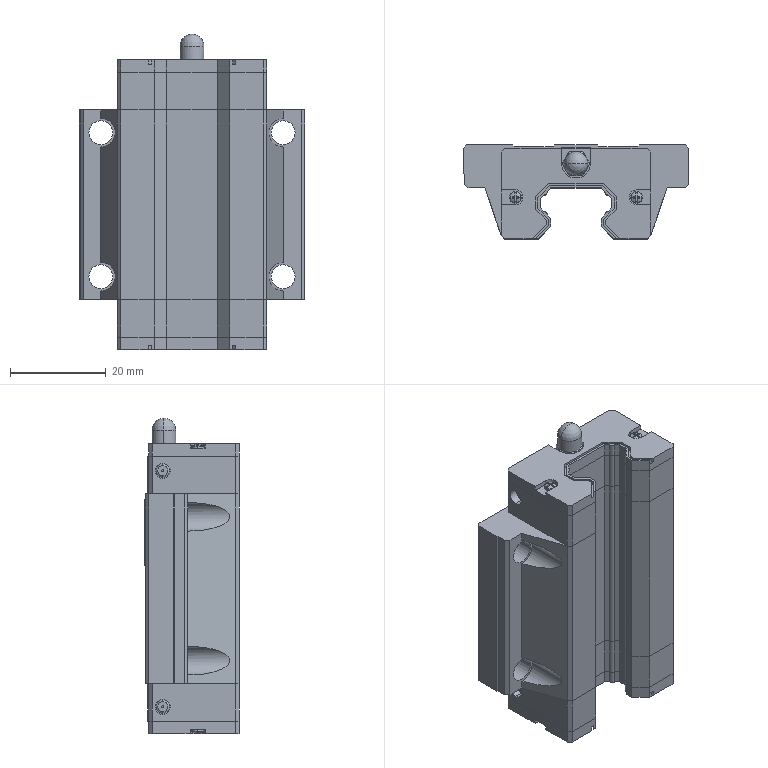Part | SolidWorks | features BaseBody 6 | 6 solids | 791 faces | box 47 x 19.61 x 65.8 mm | volume 33744 mm3 | plane 559 | spline 119 | cylinder 80 | torus 16 | sphere 10 | cone 7 | commonest cylinder face diameters 1.459 x30 3.15 x12 5 x10 0.425 x8 2.5 x8 3.125 x6